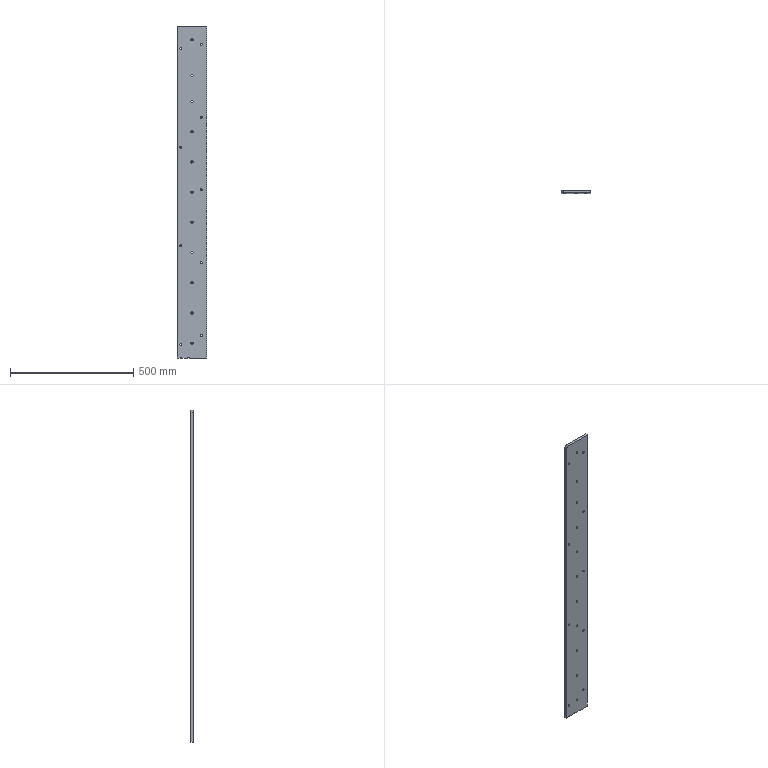Part | STEP file | 1 solid | 51 faces | box 120 x 10 x 1346 mm | volume 1602562 mm3 | cylinder 43 | plane 8 | commonest cylinder face diameters 9 x22 8.4 x10 8.5 x8 7 x2 20 x1